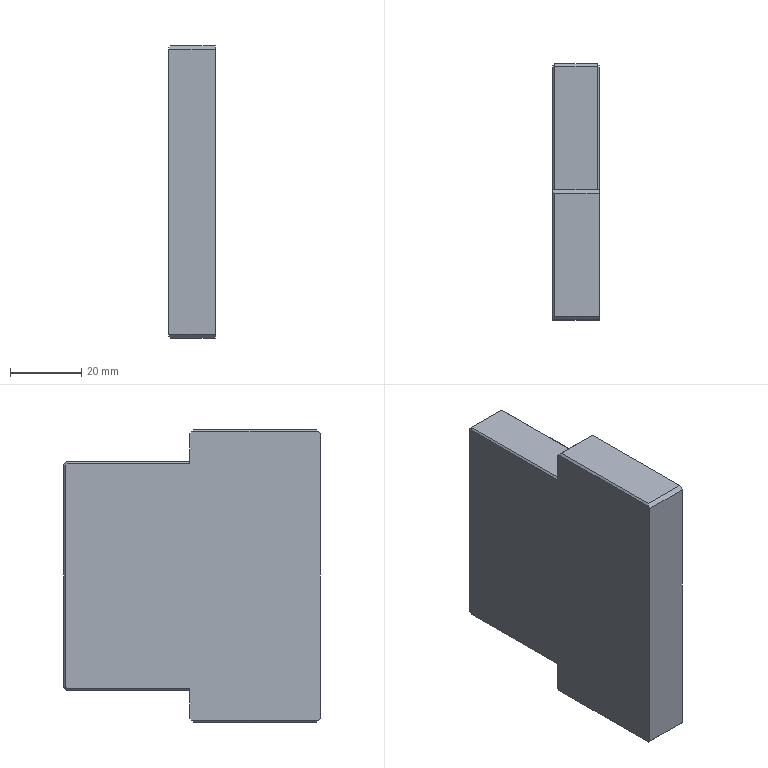Part | STEP file | 1 solid | 28 faces | box 13 x 72 x 82 mm | volume 68483 mm3 | plane 28